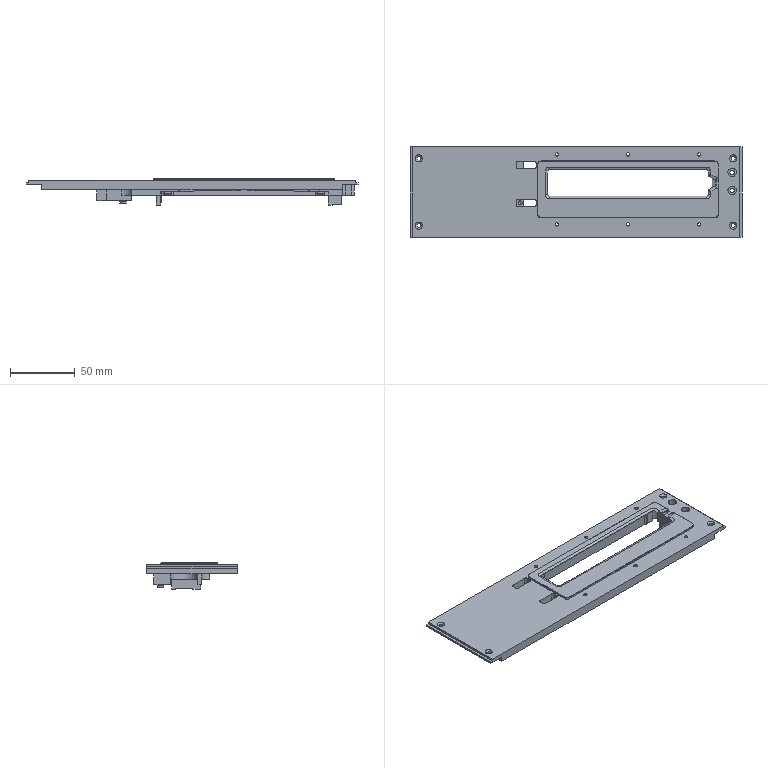NC program | NX | posted with a generic post | part box 256.6 x 70.3 x 20.422 mm
Lines 8463 to 8839 of 15201:
(DRILLING , TOOL : D6A45)
N16918 T07 M6
N16920 G54
N16922 G17 G0 G90 X-14.796 Y29. S3500 M3
N16924 G43 Z30. H7
N16926 G94 G81 G98 Z-2.4 F250. R1.6
N16928 X-43.059 Y-8.448
N16930 X-14.796 Y-25.
N16932 X40.204
N16934 Y29.
N16936 X95.204
N16938 X120.7 Y15.17
N16940 Y1.17
N16942 X95.204 Y-25.
N16944 G80
N16946 G0 X95.204 Y-25. Z30.
(DRILLING_COPY_1 , TOOL : D6A45)
N16948 X-121.5 Y26.
N16950 G81 Z-4.2 F250. R1.6
N16952 Y-26.
N16954 X121.5
N16956 Y26.
N16958 G80
N16960 G0 X121.5 Y26. Z30.
N16962 M5
(DRILLING_COPY_COPY , TOOL : 3.2ZT)
N16964 T13 M6
N16966 G54
N16968 G17 G0 G90 X-121.5 Y-26. S2500 M3
N16970 G43 Z30. H13
N16972 G94 G83 G98 Z-7.011 F120. Q2. R1.6
N16974 Y26.
N16976 X121.5 Z-6.961
N16978 Y-26.
N16980 G80
N16982 G0 X121.5 Y-26. Z30.
N16984 M5
(DRILLING_COPY_COPY_COPY , TOOL : 2.6ZT)
N16986 T12 M6
N16988 G54
N16990 G17 G0 G90 X95.204 Y-25. S2500 M3
N16992 G43 Z30. H12
N16994 G94 G83 G98 Z-10.777 F120. Q2. R1.6
N16996 Y29.
N16998 X40.204
N17000 Y-25.
N17002 X-14.796
N17004 Y29.
N17006 G80
N17008 G0 X-14.796 Y29. Z30.
N17010 M5
(DRILLING_COPY_COPY_COPY_COPY , TOOL : 3.4ZT)
N17012 T14 M6
N17014 G54
N17016 G17 G0 G90 X120.7 Y15.17 S2500 M3
N17018 G43 Z30. H14
N17020 G94 G83 G98 Z-15.221 F120. Q2. R1.6
N17022 Y1.17
N17024 G80
N17026 G0 X120.7 Y1.17 Z30.
N17028 M5
(DRILLING_COPY_COPY_COPY_COPY_COPY , TOOL : 3.1ZT)
N17030 T16 M6
N17032 G54
N17034 G17 G0 G90 X-43.059 Y-8.448 S2500 M3
N17036 G43 Z30. H16
N17038 G94 G83 G98 Z-11.001 F120. Q2. R1.6
N17040 G80
N17042 G0 X-43.059 Y-8.448 Z30.
N17044 M5
(ZLEVEL_PROFILE , TOOL : D6)
N17046 T06 M6
N17048 G54
N17050 G17 G0 G90 X96.979 Y-0.311 S9500 M3
N17052 G43 Z30. H6
N17054 Z-0.434
N17056 G94 G1 X97.153 Y-0.611 F1600.
N17058 G3 X97.672 Y-0.911 R0.6
N17060 G1 X99.857
N17062 Y0.457
N17064 G2 X99.913 Y1.153 R4.339
N17066 G3 X99.701 Y1.714 R0.6
N17068 G1 X99.473 Y1.9
N17070 G0 X96.366 Y0.4 Z-0.868
N17072 G1 X96.539 Y0.1
N17074 G3 X97.059 Y-0.2 R0.6
N17076 G1 X99.146
N17078 Y0.457
N17080 G2 X99.295 Y1.673 R5.05
N17082 G3 X99.129 Y2.25 R0.6
N17084 G1 X98.912 Y2.458
N17086 G0 X96.362 Y0.4 Z-1.302
N17088 G1 X96.535 Y0.1
N17090 G3 X97.055 Y-0.2 R0.6
N17092 G1 X99.146
N17094 Y0.457
N17096 G2 X99.295 Y1.673 R5.05
N17098 G3 X99.129 Y2.25 R0.6
N17100 G1 X98.912 Y2.458
N17102 G0 X96.362 Y0.4 Z-1.736
N17104 G1 X96.535 Y0.1
N17106 G3 X97.055 Y-0.2 R0.6
N17108 G1 X99.146
N17110 Y0.457
N17112 G2 X99.295 Y1.673 R5.05
N17114 G3 X99.129 Y2.25 R0.6
N17116 G1 X98.912 Y2.458
N17118 G0 X96.362 Y0.4 Z-2.171
N17120 G1 X96.535 Y0.1
N17122 G3 X97.055 Y-0.2 R0.6
N17124 G1 X99.146
N17126 Y0.457
N17128 G2 X99.295 Y1.673 R5.05
N17130 G3 X99.129 Y2.25 R0.6
N17132 G1 X98.912 Y2.458
N17134 G0 X96.362 Y0.4 Z-2.605
N17136 G1 X96.535 Y0.1
N17138 G3 X97.055 Y-0.2 R0.6
N17140 G1 X99.146
N17142 Y0.457
N17144 G2 X99.295 Y1.673 R5.05
N17146 G3 X99.129 Y2.25 R0.6
N17148 G1 X98.912 Y2.458
N17150 G0 X96.362 Y0.4 Z-3.039
N17152 G1 X96.535 Y0.1
N17154 G3 X97.055 Y-0.2 R0.6
N17156 G1 X99.146
N17158 Y0.457
N17160 G2 X99.295 Y1.673 R5.05
N17162 G3 X99.129 Y2.25 R0.6
N17164 G1 X98.912 Y2.458
N17166 G0 Z30.
N17168 X102.56 Y5.307
N17170 Z-0.434
N17172 G1 X102.845 Y5.139
N17174 G3 X103.445 Y5.132 R0.6
N17176 G2 X106.876 Y6.603 R17.339
N17178 G1 X106.985 Y6.683
N17180 X107.48 Y7.004
N17182 X106.894 Y7.392
N17184 G2 X103.445 Y8.868 R17.339
N17186 G3 X102.845 Y8.861 R0.6
N17188 G1 X102.56 Y8.693
N17190 G0 X101.258 Y5.304 Z-0.868
N17192 G1 X101.554 Y5.152
N17194 G3 X102.153 Y5.182 R0.6
N17196 G2 X105.82 Y7. R18.05
N17198 X102.153 Y8.818 R18.05
N17200 G3 X101.554 Y8.848 R0.6
N17202 G1 X101.258 Y8.696
N17204 G0 Y5.304 Z-1.302
N17206 G1 X101.554 Y5.152
N17208 G3 X102.153 Y5.182 R0.6
N17210 G2 X105.82 Y7. R18.05
N17212 X102.153 Y8.818 R18.05
N17214 G3 X101.554 Y8.848 R0.6
N17216 G1 X101.258 Y8.696
N17218 G0 X101.244 Y5.293 Z-1.736
N17220 G1 X101.539 Y5.142
N17222 G3 X102.138 Y5.173 R0.6
N17224 G2 X104.875 Y6.628 R18.05
N17226 G1 Y7.372
N17228 G2 X102.144 Y8.823 R18.05
N17230 G3 X101.545 Y8.854 R0.6
N17232 G1 X101.25 Y8.703
N17234 G0 X101.258 Y5.304 Z-2.171
N17236 G1 X101.554 Y5.152
N17238 G3 X102.153 Y5.182 R0.6
N17240 G2 X103.933 Y6.195 R18.05
N17242 G1 Y7.802
N17244 X103.828 Y7.856
N17246 X103.818 Y7.863
N17248 G2 X102.153 Y8.818 R18.05
N17250 G3 X101.554 Y8.848 R0.6
N17252 G1 X101.258 Y8.696
N17254 G0 X101.003 Y5.122 Z-2.605
N17256 G1 X101.301 Y4.975
N17258 G3 X101.899 Y5.015 R0.6
N17260 G2 X103.002 Y5.699 R18.05
N17262 G1 Y8.301
N17264 G2 X101.9 Y8.984 R18.05
N17266 G3 X101.301 Y9.024 R0.6
N17268 G1 X101.003 Y8.878
N17270 G0 X100.26 Y4.51 Z-3.039
N17272 G1 X100.537 Y4.395
N17274 G3 X101.132 Y4.471 R0.6
N17276 G1 X101.184 Y4.51
N17278 G2 X102.14 Y5.174 R18.05
N17280 G1 Y6.443
N17282 G3 X101.84 Y6.963 R0.6
N17284 G1 X101.54 Y7.136
N17286 G0 Z30.
N17288 Y6.864
N17290 Z-3.039
N17292 G1 X101.84 Y7.037
N17294 G3 X102.14 Y7.557 R0.6
N17296 G1 Y8.826
N17298 G2 X101.184 Y9.49 R18.05
N17300 G1 X101.132 Y9.529
N17302 G3 X100.537 Y9.605 R0.6
N17304 G1 X100.26 Y9.49
N17306 G0 Z30.
N17308 X99.473 Y12.1
N17310 Z-0.434
N17312 G1 X99.701 Y12.286
N17314 G3 X99.913 Y12.847 R0.6
N17316 G2 X99.857 Y13.543 R4.339
N17318 G1 Y14.911
N17320 X97.672
N17322 G3 X97.153 Y14.611 R0.6
N17324 G1 X96.979 Y14.311
N17326 G0 X98.912 Y11.542 Z-0.868
N17328 G1 X99.129 Y11.75
N17330 G3 X99.295 Y12.327 R0.6
N17332 G2 X99.146 Y13.543 R5.05
N17334 G1 Y14.2
N17336 X97.059
N17338 G3 X96.539 Y13.9 R0.6
N17340 G1 X96.366 Y13.6
N17342 G0 X98.913 Y11.539 Z-1.302
N17344 G1 X99.129 Y11.748
N17346 G3 X99.295 Y12.325 R0.6
N17348 G2 X99.146 Y13.543 R5.05
N17350 G1 Y14.2
N17352 X97.065
N17354 G3 X96.546 Y13.9 R0.6
N17356 G1 X96.373 Y13.6
N17358 G0 X98.913 Y11.539 Z-1.736
N17360 G1 X99.129 Y11.748
N17362 G3 X99.295 Y12.325 R0.6
N17364 G2 X99.146 Y13.543 R5.05
N17366 G1 Y14.2
N17368 X97.065
N17370 G3 X96.546 Y13.9 R0.6
N17372 G1 X96.373 Y13.6
N17374 G0 X98.913 Y11.539 Z-2.171
N17376 G1 X99.129 Y11.748
N17378 G3 X99.295 Y12.325 R0.6
N17380 G2 X99.146 Y13.543 R5.05
N17382 G1 Y14.2
N17384 X97.065
N17386 G3 X96.546 Y13.9 R0.6
N17388 G1 X96.373 Y13.6
N17390 G0 X98.913 Y11.539 Z-2.605
N17392 G1 X99.129 Y11.748
N17394 G3 X99.295 Y12.325 R0.6
N17396 G2 X99.146 Y13.543 R5.05
N17398 G1 Y14.2
N17400 X97.065
N17402 G3 X96.546 Y13.9 R0.6
N17404 G1 X96.373 Y13.6
N17406 G0 X98.913 Y11.539 Z-3.039
N17408 G1 X99.129 Y11.748
N17410 G3 X99.295 Y12.325 R0.6
N17412 G2 X99.146 Y13.543 R5.05
N17414 G1 Y14.2
N17416 X97.065
N17418 G3 X96.546 Y13.9 R0.6
N17420 G1 X96.373 Y13.6
N17422 G0 Z30.
N17424 X-16.556 Y14.311
N17426 Z-0.434
N17428 G1 X-16.729 Y14.611
N17430 G3 X-17.249 Y14.911 R0.6
N17432 G1 X-19.465
N17434 Y12.695
N17436 G3 X-19.165 Y12.175 R0.6
N17438 G1 X-18.865 Y12.002
N17440 G0 X-15.845 Y13.6 Z-0.868
N17442 G1 X-16.018 Y13.9
N17444 G3 X-16.538 Y14.2 R0.6
N17446 G1 X-18.754
N17448 Y11.984
N17450 G3 X-18.454 Y11.464 R0.6
N17452 G1 X-18.154 Y11.291
N17454 G0 X-15.854 Y13.6 Z-1.302
N17456 G1 X-16.027 Y13.9
N17458 G3 X-16.547 Y14.2 R0.6
N17460 G1 X-18.754
N17462 Y11.99
N17464 G3 X-18.454 Y11.47 R0.6
N17466 G1 X-18.154 Y11.297
N17468 G0 X-15.854 Y13.6 Z-1.736
N17470 G1 X-16.027 Y13.9
N17472 G3 X-16.547 Y14.2 R0.6
N17474 G1 X-18.754
N17476 Y11.99
N17478 G3 X-18.454 Y11.47 R0.6
N17480 G1 X-18.154 Y11.297
N17482 G0 X-15.854 Y13.6 Z-2.171
N17484 G1 X-16.027 Y13.9
N17486 G3 X-16.547 Y14.2 R0.6
N17488 G1 X-18.754
N17490 Y11.99
N17492 G3 X-18.454 Y11.47 R0.6
N17494 G1 X-18.154 Y11.297
N17496 G0 X-15.854 Y13.6 Z-2.605
N17498 G1 X-16.027 Y13.9
N17500 G3 X-16.547 Y14.2 R0.6
N17502 G1 X-18.754
N17504 Y11.99
N17506 G3 X-18.454 Y11.47 R0.6
N17508 G1 X-18.154 Y11.297
N17510 G0 X-15.854 Y13.6 Z-3.039
N17512 G1 X-16.027 Y13.9
N17514 G3 X-16.547 Y14.2 R0.6
N17516 G1 X-18.754
N17518 Y11.99
N17520 G3 X-18.454 Y11.47 R0.6
N17522 G1 X-18.154 Y11.297
N17524 G0 Z30.
N17526 X-18.865 Y1.998
N17528 Z-0.434
N17530 G1 X-19.165 Y1.825
N17532 G3 X-19.465 Y1.305 R0.6
N17534 G1 Y-0.911
N17536 X-17.249
N17538 G3 X-16.729 Y-0.611 R0.6
N17540 G1 X-16.556 Y-0.311
N17542 G0 X-18.154 Y2.709 Z-0.868
N17544 G1 X-18.454 Y2.536
N17546 G3 X-18.754 Y2.016 R0.6
N17548 G1 Y-0.2
N17550 X-16.538
N17552 G3 X-16.018 Y0.1 R0.6
N17554 G1 X-15.845 Y0.4
N17556 G0 X-18.154 Y2.709 Z-1.302
N17558 G1 X-18.454 Y2.536
N17560 G3 X-18.754 Y2.016 R0.6
N17562 G1 Y-0.2
N17564 X-16.538
N17566 G3 X-16.018 Y0.1 R0.6
N17568 G1 X-15.845 Y0.4
N17570 G0 X-18.154 Y2.709 Z-1.736
N17572 G1 X-18.454 Y2.536
N17574 G3 X-18.754 Y2.016 R0.6
N17576 G1 Y-0.2
N17578 X-16.538
N17580 G3 X-16.018 Y0.1 R0.6
N17582 G1 X-15.845 Y0.4
N17584 G0 X-18.154 Y2.709 Z-2.171
N17586 G1 X-18.454 Y2.536
N17588 G3 X-18.754 Y2.016 R0.6
N17590 G1 Y-0.2
N17592 X-16.538
N17594 G3 X-16.018 Y0.1 R0.6
N17596 G1 X-15.845 Y0.4
N17598 G0 X-18.154 Y2.709 Z-2.605
N17600 G1 X-18.454 Y2.536
N17602 G3 X-18.754 Y2.016 R0.6
N17604 G1 Y-0.2
N17606 X-16.538
N17608 G3 X-16.018 Y0.1 R0.6
N17610 G1 X-15.845 Y0.4
N17612 G0 X-18.154 Y2.709 Z-3.039
N17614 G1 X-18.454 Y2.536
N17616 G3 X-18.754 Y2.016 R0.6
N17618 G1 Y-0.2
N17620 X-16.538
N17622 G3 X-16.018 Y0.1 R0.6
N17624 G1 X-15.845 Y0.4
N17626 G0 Z30.
N17628 M5